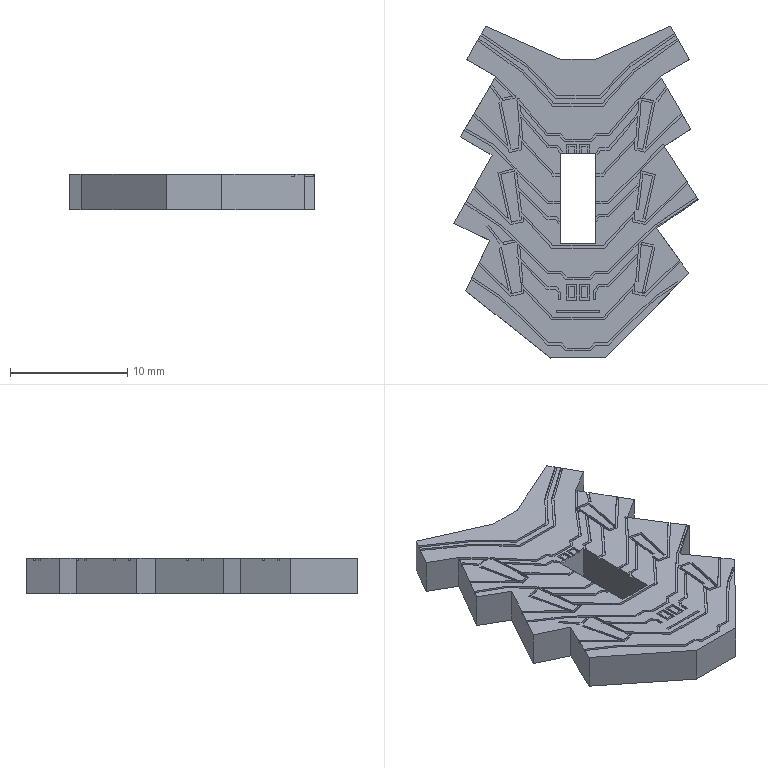Part | SolidWorks | features BaseBody 1 | 1 solid | 434 faces | box 20.837 x 28.283 x 3 mm | volume 1191 mm3 | plane 433 | spline 1